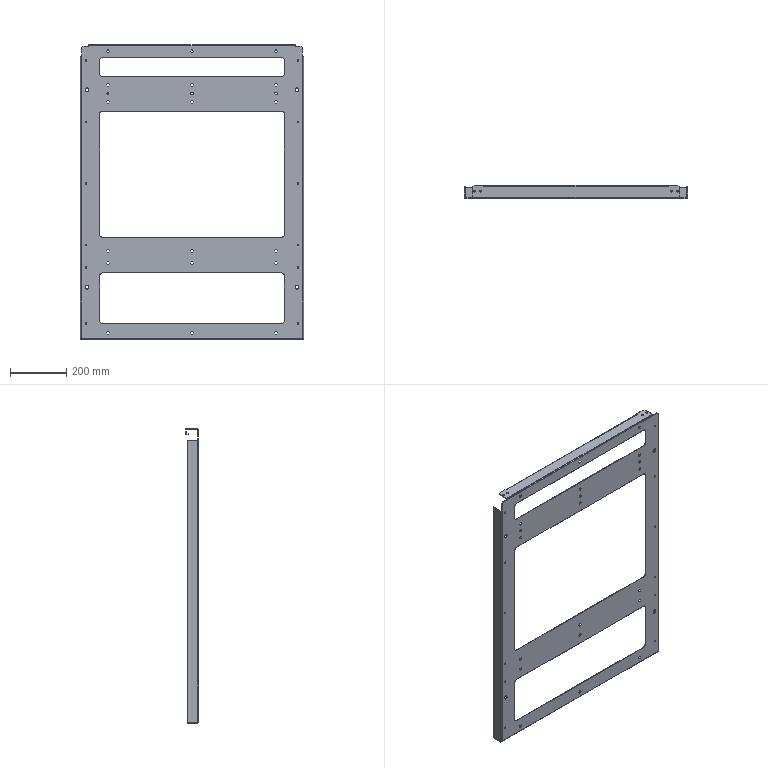Part | STEP file | 1 solid | 258 faces | box 796 x 45 x 1050 mm | volume 1045363 mm3 | plane 182 | cylinder 76 | commonest cylinder face diameters 5.3 x24 7 x16 20.5 x12 13 x8 3 x6 4.2 x6